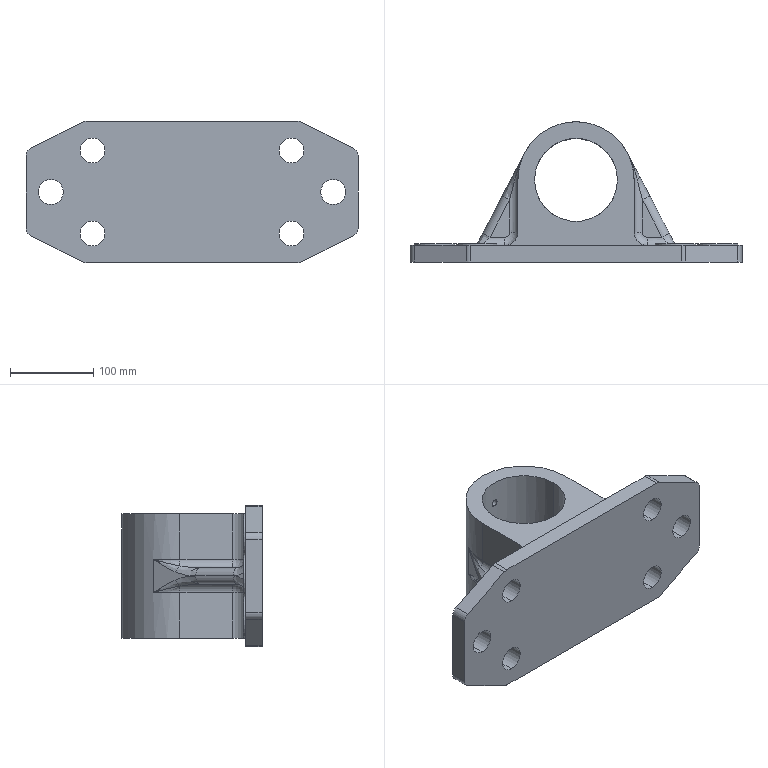Part | SolidWorks | features MirrorStock 1 | 1 solid | 125 faces | box 400 x 169 x 170 mm | volume 2936376 mm3 | cylinder 64 | plane 30 | spline 12 | cone 11 | torus 8 | commonest cylinder face diameters 20 x20 30 x12 50 x12 8.5 x10 32 x4 6.8 x3